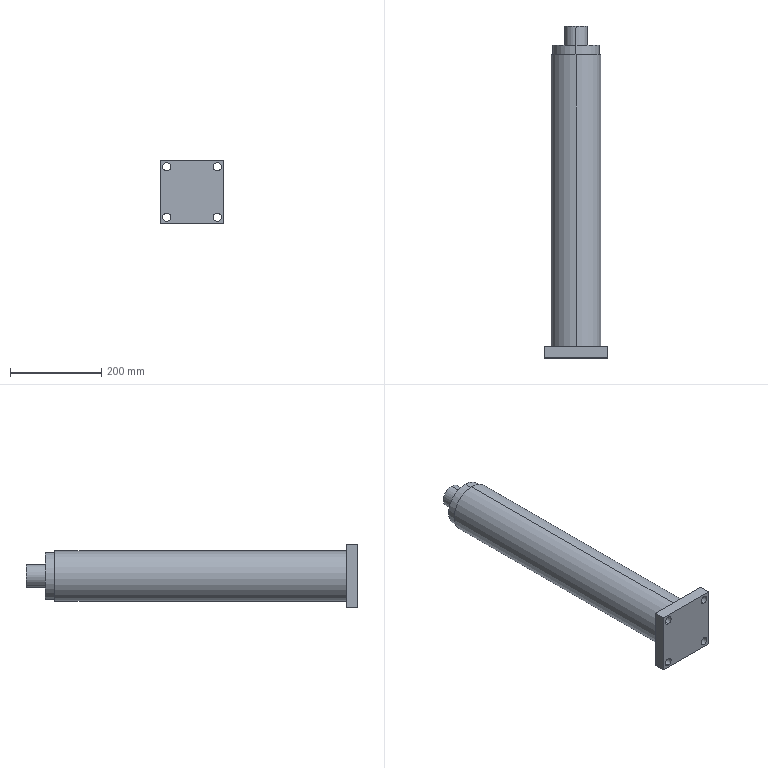Part | SolidWorks | features ICE 1, Revolution 1 | 1 solid | 23 faces | box 140 x 729 x 140 mm | volume 6809578 mm3 | cylinder 14 | plane 9 | commonest cylinder face diameters 18 x8 50 x2 102 x2 110 x2
STEP:
#1=CARTESIAN_POINT('',(-55.5,25.,46.5));
#2=VERTEX_POINT('',#1);
#3=CARTESIAN_POINT('',(-55.5,25.,64.5));
#4=VERTEX_POINT('',#3);
#5=CARTESIAN_POINT('',(-55.5,25.,55.5));
#6=DIRECTION('',(0.,1.,0.));
#7=DIRECTION('',(0.,0.,1.));
#8=AXIS2_PLACEMENT_3D('',#5,#6,#7);
#9=CIRCLE('',#8,9.);
#10=EDGE_CURVE('',#2,#4,#9,.T.);
#11=ORIENTED_EDGE('',*,*,#10,.T.);
#12=CARTESIAN_POINT('',(-55.5,0.,64.5));
#13=VERTEX_POINT('',#12);
#14=CARTESIAN_POINT('',(-55.5,25.,64.5));
#15=DIRECTION('',(0.,-1.,0.));
#16=VECTOR('',#15,1000.);
#17=LINE('',#14,#16);
#18=EDGE_CURVE('',#4,#13,#17,.T.);
#19=ORIENTED_EDGE('',*,*,#18,.T.);
#20=CARTESIAN_POINT('',(-55.5,0.,46.5));
#21=VERTEX_POINT('',#20);
#22=CARTESIAN_POINT('',(-55.5,0.,55.5));
#23=DIRECTION('',(0.,1.,0.));
#24=DIRECTION('',(0.,0.,1.));
#25=AXIS2_PLACEMENT_3D('',#22,#23,#24);
#26=CIRCLE('',#25,9.);
#27=EDGE_CURVE('',#21,#13,#26,.T.);
#28=ORIENTED_EDGE('',*,*,#27,.F.);
#29=CARTESIAN_POINT('',(-55.5,25.,46.5));
#30=DIRECTION('',(0.,-1.,0.));
#31=VECTOR('',#30,1000.);
#32=LINE('',#29,#31);
#33=EDGE_CURVE('',#2,#21,#32,.T.);
#34=ORIENTED_EDGE('',*,*,#33,.F.);
#35=EDGE_LOOP('',(#11,#19,#28,#34));
#36=FACE_OUTER_BOUND('',#35,.T.);
#37=CARTESIAN_POINT('',(-55.5,25.,55.5));
#38=DIRECTION('',(0.,-1.,0.));
#39=DIRECTION('',(0.,0.,-1.));
#40=AXIS2_PLACEMENT_3D('',#37,#38,#39);
#41=CYLINDRICAL_SURFACE('',#40,9.);
#42=ADVANCED_FACE('',(#36),#41,.F.);
#43=CARTESIAN_POINT('',(55.5,25.,46.5));
#44=VERTEX_POINT('',#43);
#45=CARTESIAN_POINT('',(55.5,25.,64.5));
#46=VERTEX_POINT('',#45);
#47=CARTESIAN_POINT('',(55.5,25.,55.5));
#48=DIRECTION('',(0.,1.,0.));
#49=DIRECTION('',(0.,0.,1.));
#50=AXIS2_PLACEMENT_3D('',#47,#48,#49);
#51=CIRCLE('',#50,9.);
#52=EDGE_CURVE('',#44,#46,#51,.T.);
#53=ORIENTED_EDGE('',*,*,#52,.T.);
#54=CARTESIAN_POINT('',(55.5,0.,64.5));
#55=VERTEX_POINT('',#54);
#56=CARTESIAN_POINT('',(55.5,25.,64.5));
#57=DIRECTION('',(0.,-1.,0.));
#58=VECTOR('',#57,1000.);
#59=LINE('',#56,#58);
#60=EDGE_CURVE('',#46,#55,#59,.T.);
#61=ORIENTED_EDGE('',*,*,#60,.T.);
#62=CARTESIAN_POINT('',(55.5,0.,46.5));
#63=VERTEX_POINT('',#62);
#64=CARTESIAN_POINT('',(55.5,0.,55.5));
#65=DIRECTION('',(0.,1.,0.));
#66=DIRECTION('',(0.,0.,1.));
#67=AXIS2_PLACEMENT_3D('',#64,#65,#66);
#68=CIRCLE('',#67,9.);
#69=EDGE_CURVE('',#63,#55,#68,.T.);
#70=ORIENTED_EDGE('',*,*,#69,.F.);
#71=CARTESIAN_POINT('',(55.5,25.,46.5));
#72=DIRECTION('',(0.,-1.,0.));
#73=VECTOR('',#72,1000.);
#74=LINE('',#71,#73);
#75=EDGE_CURVE('',#44,#63,#74,.T.);
#76=ORIENTED_EDGE('',*,*,#75,.F.);
#77=EDGE_LOOP('',(#53,#61,#70,#76));
#78=FACE_OUTER_BOUND('',#77,.T.);
#79=CARTESIAN_POINT('',(55.5,25.,55.5));
#80=DIRECTION('',(0.,-1.,0.));
#81=DIRECTION('',(0.,0.,-1.));
#82=AXIS2_PLACEMENT_3D('',#79,#80,#81);
#83=CYLINDRICAL_SURFACE('',#82,9.);
#84=ADVANCED_FACE('',(#78),#83,.F.);
#85=CARTESIAN_POINT('',(55.5,25.,-64.5));
#86=VERTEX_POINT('',#85);
#87=CARTESIAN_POINT('',(55.5,25.,-46.5));
#88=VERTEX_POINT('',#87);
#89=CARTESIAN_POINT('',(55.5,25.,-55.5));
#90=DIRECTION('',(0.,1.,0.));
#91=DIRECTION('',(0.,0.,1.));
#92=AXIS2_PLACEMENT_3D('',#89,#90,#91);
#93=CIRCLE('',#92,9.);
#94=EDGE_CURVE('',#86,#88,#93,.T.);
#95=ORIENTED_EDGE('',*,*,#94,.T.);
#96=CARTESIAN_POINT('',(55.5,0.,-46.5));
#97=VERTEX_POINT('',#96);
#98=CARTESIAN_POINT('',(55.5,25.,-46.5));
#99=DIRECTION('',(0.,-1.,0.));
#100=VECTOR('',#99,1000.);
#101=LINE('',#98,#100);
#102=EDGE_CURVE('',#88,#97,#101,.T.);
#103=ORIENTED_EDGE('',*,*,#102,.T.);
#104=CARTESIAN_POINT('',(55.5,0.,-64.5));
#105=VERTEX_POINT('',#104);
#106=CARTESIAN_POINT('',(55.5,0.,-55.5));
#107=DIRECTION('',(0.,1.,0.));
#108=DIRECTION('',(0.,0.,1.));
#109=AXIS2_PLACEMENT_3D('',#106,#107,#108);
#110=CIRCLE('',#109,9.);
#111=EDGE_CURVE('',#105,#97,#110,.T.);
#112=ORIENTED_EDGE('',*,*,#111,.F.);
#113=CARTESIAN_POINT('',(55.5,25.,-64.5));
#114=DIRECTION('',(0.,-1.,0.));
#115=VECTOR('',#114,1000.);
#116=LINE('',#113,#115);
#117=EDGE_CURVE('',#86,#105,#116,.T.);
#118=ORIENTED_EDGE('',*,*,#117,.F.);
#119=EDGE_LOOP('',(#95,#103,#112,#118));
#120=FACE_OUTER_BOUND('',#119,.T.);
#121=CARTESIAN_POINT('',(55.5,25.,-55.5));
#122=DIRECTION('',(0.,-1.,0.));
#123=DIRECTION('',(0.,0.,-1.));
#124=AXIS2_PLACEMENT_3D('',#121,#122,#123);
#125=CYLINDRICAL_SURFACE('',#124,9.);
#126=ADVANCED_FACE('',(#120),#125,.F.);
#127=CARTESIAN_POINT('',(-55.5,25.,-64.5));
#128=VERTEX_POINT('',#127);
#129=CARTESIAN_POINT('',(-55.5,25.,-46.5));
#130=VERTEX_POINT('',#129);
#131=CARTESIAN_POINT('',(-55.5,25.,-55.5));
#132=DIRECTION('',(0.,1.,0.));
#133=DIRECTION('',(0.,0.,1.));
#134=AXIS2_PLACEMENT_3D('',#131,#132,#133);
#135=CIRCLE('',#134,9.);
#136=EDGE_CURVE('',#128,#130,#135,.T.);
#137=ORIENTED_EDGE('',*,*,#136,.T.);
#138=CARTESIAN_POINT('',(-55.5,0.,-46.5));
#139=VERTEX_POINT('',#138);
#140=CARTESIAN_POINT('',(-55.5,25.,-46.5));
#141=DIRECTION('',(0.,-1.,0.));
#142=VECTOR('',#141,1000.);
#143=LINE('',#140,#142);
#144=EDGE_CURVE('',#130,#139,#143,.T.);
#145=ORIENTED_EDGE('',*,*,#144,.T.);
#146=CARTESIAN_POINT('',(-55.5,0.,-64.5));
#147=VERTEX_POINT('',#146);
#148=CARTESIAN_POINT('',(-55.5,0.,-55.5));
#149=DIRECTION('',(0.,1.,0.));
#150=DIRECTION('',(0.,0.,1.));
#151=AXIS2_PLACEMENT_3D('',#148,#149,#150);
#152=CIRCLE('',#151,9.);
#153=EDGE_CURVE('',#147,#139,#152,.T.);
#154=ORIENTED_EDGE('',*,*,#153,.F.);
#155=CARTESIAN_POINT('',(-55.5,25.,-64.5));
#156=DIRECTION('',(0.,-1.,0.));
#157=VECTOR('',#156,1000.);
#158=LINE('',#155,#157);
#159=EDGE_CURVE('',#128,#147,#158,.T.);
#160=ORIENTED_EDGE('',*,*,#159,.F.);
#161=EDGE_LOOP('',(#137,#145,#154,#160));
#162=FACE_OUTER_BOUND('',#161,.T.);
#163=CARTESIAN_POINT('',(-55.5,25.,-55.5));
#164=DIRECTION('',(0.,-1.,0.));
#165=DIRECTION('',(0.,0.,-1.));
#166=AXIS2_PLACEMENT_3D('',#163,#164,#165);
#167=CYLINDRICAL_SURFACE('',#166,9.);
#168=ADVANCED_FACE('',(#162),#167,.F.);
#169=CARTESIAN_POINT('',(0.,687.,25.));
#170=VERTEX_POINT('',#169);
#171=CARTESIAN_POINT('',(0.,687.,-25.));
#172=VERTEX_POINT('',#171);
#173=CARTESIAN_POINT('',(0.,687.,0.));
#174=DIRECTION('',(0.,1.,0.));
#175=DIRECTION('',(0.,0.,1.));
#176=AXIS2_PLACEMENT_3D('',#173,#174,#175);
#177=CIRCLE('',#176,25.);
#178=EDGE_CURVE('',#170,#172,#177,.T.);
#179=ORIENTED_EDGE('',*,*,#178,.T.);
#180=CARTESIAN_POINT('',(0.,729.,-25.));
#181=VERTEX_POINT('',#180);
#182=CARTESIAN_POINT('',(0.,0.,-25.));
#183=DIRECTION('',(0.,1.,0.));
#184=VECTOR('',#183,1000.);
#185=LINE('',#182,#184);
#186=EDGE_CURVE('',#172,#181,#185,.T.);
#187=ORIENTED_EDGE('',*,*,#186,.T.);
#188=CARTESIAN_POINT('',(0.,729.,25.));
#189=VERTEX_POINT('',#188);
#190=CARTESIAN_POINT('',(0.,729.,0.));
#191=DIRECTION('',(0.,1.,0.));
#192=DIRECTION('',(0.,0.,1.));
#193=AXIS2_PLACEMENT_3D('',#190,#191,#192);
#194=CIRCLE('',#193,25.);
#195=EDGE_CURVE('',#189,#181,#194,.T.);
#196=ORIENTED_EDGE('',*,*,#195,.F.);
#197=CARTESIAN_POINT('',(0.,0.,25.));
#198=DIRECTION('',(0.,1.,0.));
#199=VECTOR('',#198,1000.);
#200=LINE('',#197,#199);
#201=EDGE_CURVE('',#170,#189,#200,.T.);
#202=ORIENTED_EDGE('',*,*,#201,.F.);
#203=EDGE_LOOP('',(#179,#187,#196,#202));
#204=FACE_OUTER_BOUND('',#203,.T.);
#205=CARTESIAN_POINT('',(0.,0.,0.));
#206=DIRECTION('',(0.,1.,0.));
#207=DIRECTION('',(0.,0.,1.));
#208=AXIS2_PLACEMENT_3D('',#205,#206,#207);
#209=CYLINDRICAL_SURFACE('',#208,25.);
#210=ADVANCED_FACE('',(#204),#209,.T.);
#211=CARTESIAN_POINT('',(0.,665.5,51.));
#212=VERTEX_POINT('',#211);
#213=CARTESIAN_POINT('',(0.,665.5,-51.));
#214=VERTEX_POINT('',#213);
#215=CARTESIAN_POINT('',(0.,665.5,0.));
#216=DIRECTION('',(0.,1.,0.));
#217=DIRECTION('',(0.,0.,1.));
#218=AXIS2_PLACEMENT_3D('',#215,#216,#217);
#219=CIRCLE('',#218,51.);
#220=EDGE_CURVE('',#212,#214,#219,.T.);
#221=ORIENTED_EDGE('',*,*,#220,.T.);
#222=CARTESIAN_POINT('',(0.,687.,-51.));
#223=VERTEX_POINT('',#222);
#224=CARTESIAN_POINT('',(0.,0.,-51.));
#225=DIRECTION('',(0.,1.,0.));
#226=VECTOR('',#225,1000.);
#227=LINE('',#224,#226);
#228=EDGE_CURVE('',#214,#223,#227,.T.);
#229=ORIENTED_EDGE('',*,*,#228,.T.);
#230=CARTESIAN_POINT('',(0.,687.,51.));
#231=VERTEX_POINT('',#230);
#232=CARTESIAN_POINT('',(0.,687.,0.));
#233=DIRECTION('',(0.,1.,0.));
#234=DIRECTION('',(0.,0.,1.));
#235=AXIS2_PLACEMENT_3D('',#232,#233,#234);
#236=CIRCLE('',#235,51.);
#237=EDGE_CURVE('',#231,#223,#236,.T.);
#238=ORIENTED_EDGE('',*,*,#237,.F.);
#239=CARTESIAN_POINT('',(0.,0.,51.));
#240=DIRECTION('',(0.,1.,0.));
#241=VECTOR('',#240,1000.);
#242=LINE('',#239,#241);
#243=EDGE_CURVE('',#212,#231,#242,.T.);
#244=ORIENTED_EDGE('',*,*,#243,.F.);
#245=EDGE_LOOP('',(#221,#229,#238,#244));
#246=FACE_OUTER_BOUND('',#245,.T.);
#247=CARTESIAN_POINT('',(0.,0.,0.));
#248=DIRECTION('',(0.,1.,0.));
#249=DIRECTION('',(0.,0.,1.));
#250=AXIS2_PLACEMENT_3D('',#247,#248,#249);
#251=CYLINDRICAL_SURFACE('',#250,51.);
#252=ADVANCED_FACE('',(#246),#251,.T.);
#253=CARTESIAN_POINT('',(0.,25.,55.));
#254=VERTEX_POINT('',#253);
#255=CARTESIAN_POINT('',(0.,25.,-55.));
#256=VERTEX_POINT('',#255);
#257=CARTESIAN_POINT('',(0.,25.,0.));
#258=DIRECTION('',(0.,1.,0.));
#259=DIRECTION('',(0.,0.,1.));
#260=AXIS2_PLACEMENT_3D('',#257,#258,#259);
#261=CIRCLE('',#260,55.);
#262=EDGE_CURVE('',#254,#256,#261,.T.);
#263=ORIENTED_EDGE('',*,*,#262,.T.);
#264=CARTESIAN_POINT('',(0.,665.5,-55.));
#265=VERTEX_POINT('',#264);
#266=CARTESIAN_POINT('',(0.,0.,-55.));
#267=DIRECTION('',(0.,1.,0.));
#268=VECTOR('',#267,1000.);
#269=LINE('',#266,#268);
#270=EDGE_CURVE('',#256,#265,#269,.T.);
#271=ORIENTED_EDGE('',*,*,#270,.T.);
#272=CARTESIAN_POINT('',(0.,665.5,55.));
#273=VERTEX_POINT('',#272);
#274=CARTESIAN_POINT('',(0.,665.5,0.));
#275=DIRECTION('',(0.,1.,0.));
#276=DIRECTION('',(0.,0.,1.));
#277=AXIS2_PLACEMENT_3D('',#274,#275,#276);
#278=CIRCLE('',#277,55.);
#279=EDGE_CURVE('',#273,#265,#278,.T.);
#280=ORIENTED_EDGE('',*,*,#279,.F.);
#281=CARTESIAN_POINT('',(0.,0.,55.));
#282=DIRECTION('',(0.,1.,0.));
#283=VECTOR('',#282,1000.);
#284=LINE('',#281,#283);
#285=EDGE_CURVE('',#254,#273,#284,.T.);
#286=ORIENTED_EDGE('',*,*,#285,.F.);
#287=EDGE_LOOP('',(#263,#271,#280,#286));
#288=FACE_OUTER_BOUND('',#287,.T.);
#289=CARTESIAN_POINT('',(0.,0.,0.));
#290=DIRECTION('',(0.,1.,0.));
#291=DIRECTION('',(0.,0.,1.));
#292=AXIS2_PLACEMENT_3D('',#289,#290,#291);
#293=CYLINDRICAL_SURFACE('',#292,55.);
#294=ADVANCED_FACE('',(#288),#293,.T.);
#295=ORIENTED_EDGE('',*,*,#262,.F.);
#296=CARTESIAN_POINT('',(0.,25.,0.));
#297=DIRECTION('',(0.,1.,0.));
#298=DIRECTION('',(0.,0.,1.));
#299=AXIS2_PLACEMENT_3D('',#296,#297,#298);
#300=CIRCLE('',#299,55.);
#301=EDGE_CURVE('',#256,#254,#300,.T.);
#302=ORIENTED_EDGE('',*,*,#301,.F.);
#303=EDGE_LOOP('',(#295,#302));
#304=FACE_BOUND('',#303,.T.);
#305=ORIENTED_EDGE('',*,*,#52,.F.);
#306=CARTESIAN_POINT('',(55.5,25.,55.5));
#307=DIRECTION('',(0.,1.,0.));
#308=DIRECTION('',(0.,0.,1.));
#309=AXIS2_PLACEMENT_3D('',#306,#307,#308);
#310=CIRCLE('',#309,9.);
#311=EDGE_CURVE('',#46,#44,#310,.T.);
#312=ORIENTED_EDGE('',*,*,#311,.F.);
#313=EDGE_LOOP('',(#305,#312));
#314=FACE_BOUND('',#313,.T.);
#315=ORIENTED_EDGE('',*,*,#136,.F.);
#316=CARTESIAN_POINT('',(-55.5,25.,-55.5));
#317=DIRECTION('',(0.,1.,0.));
#318=DIRECTION('',(0.,0.,1.));
#319=AXIS2_PLACEMENT_3D('',#316,#317,#318);
#320=CIRCLE('',#319,9.);
#321=EDGE_CURVE('',#130,#128,#320,.T.);
#322=ORIENTED_EDGE('',*,*,#321,.F.);
#323=EDGE_LOOP('',(#315,#322));
#324=FACE_BOUND('',#323,.T.);
#325=CARTESIAN_POINT('',(-70.,25.,-70.));
#326=VERTEX_POINT('',#325);
#327=CARTESIAN_POINT('',(-70.,25.,70.));
#328=VERTEX_POINT('',#327);
#329=CARTESIAN_POINT('',(-70.,25.,70.));
#330=DIRECTION('',(0.,0.,1.));
#331=VECTOR('',#330,1000.);
#332=LINE('',#329,#331);
#333=EDGE_CURVE('',#326,#328,#332,.T.);
#334=ORIENTED_EDGE('',*,*,#333,.T.);
#335=CARTESIAN_POINT('',(70.,25.,70.));
#336=VERTEX_POINT('',#335);
#337=CARTESIAN_POINT('',(70.,25.,70.));
#338=DIRECTION('',(1.,0.,0.));
#339=VECTOR('',#338,1000.);
#340=LINE('',#337,#339);
#341=EDGE_CURVE('',#328,#336,#340,.T.);
#342=ORIENTED_EDGE('',*,*,#341,.T.);
#343=CARTESIAN_POINT('',(70.,25.,-70.));
#344=VERTEX_POINT('',#343);
#345=CARTESIAN_POINT('',(70.,25.,70.));
#346=DIRECTION('',(0.,0.,-1.));
#347=VECTOR('',#346,1000.);
#348=LINE('',#345,#347);
#349=EDGE_CURVE('',#336,#344,#348,.T.);
#350=ORIENTED_EDGE('',*,*,#349,.T.);
#351=CARTESIAN_POINT('',(70.,25.,-70.));
#352=DIRECTION('',(-1.,0.,0.));
#353=VECTOR('',#352,1000.);
#354=LINE('',#351,#353);
#355=EDGE_CURVE('',#344,#326,#354,.T.);
#356=ORIENTED_EDGE('',*,*,#355,.T.);
#357=EDGE_LOOP('',(#334,#342,#350,#356));
#358=FACE_OUTER_BOUND('',#357,.T.);
#359=ORIENTED_EDGE('',*,*,#94,.F.);
#360=CARTESIAN_POINT('',(55.5,25.,-55.5));
#361=DIRECTION('',(0.,1.,0.));
#362=DIRECTION('',(0.,0.,1.));
#363=AXIS2_PLACEMENT_3D('',#360,#361,#362);
#364=CIRCLE('',#363,9.);
#365=EDGE_CURVE('',#88,#86,#364,.T.);
#366=ORIENTED_EDGE('',*,*,#365,.F.);
#367=EDGE_LOOP('',(#359,#366));
#368=FACE_BOUND('',#367,.T.);
#369=ORIENTED_EDGE('',*,*,#10,.F.);
#370=CARTESIAN_POINT('',(-55.5,25.,55.5));
#371=DIRECTION('',(0.,1.,0.));
#372=DIRECTION('',(0.,0.,1.));
#373=AXIS2_PLACEMENT_3D('',#370,#371,#372);
#374=CIRCLE('',#373,9.);
#375=EDGE_CURVE('',#4,#2,#374,.T.);
#376=ORIENTED_EDGE('',*,*,#375,.F.);
#377=EDGE_LOOP('',(#369,#376));
#378=FACE_BOUND('',#377,.T.);
#379=CARTESIAN_POINT('',(60.,25.,0.));
#380=DIRECTION('',(0.,-1.,0.));
#381=DIRECTION('',(0.,0.,-1.));
#382=AXIS2_PLACEMENT_3D('',#379,#380,#381);
#383=PLANE('',#382);
#384=ADVANCED_FACE('',(#304,#314,#324,#358,#368,#378),#383,.F.);
#385=ORIENTED_EDGE('',*,*,#270,.F.);
#386=ORIENTED_EDGE('',*,*,#301,.T.);
#387=ORIENTED_EDGE('',*,*,#285,.T.);
#388=CARTESIAN_POINT('',(0.,665.5,0.));
#389=DIRECTION('',(0.,1.,0.));
#390=DIRECTION('',(0.,0.,1.));
#391=AXIS2_PLACEMENT_3D('',#388,#389,#390);
#392=CIRCLE('',#391,55.);
#393=EDGE_CURVE('',#265,#273,#392,.T.);
#394=ORIENTED_EDGE('',*,*,#393,.F.);
#395=EDGE_LOOP('',(#385,#386,#387,#394));
#396=FACE_OUTER_BOUND('',#395,.T.);
#397=CARTESIAN_POINT('',(0.,0.,0.));
#398=DIRECTION('',(0.,1.,0.));
#399=DIRECTION('',(0.,0.,1.));
#400=AXIS2_PLACEMENT_3D('',#397,#398,#399);
#401=CYLINDRICAL_SURFACE('',#400,55.);
#402=ADVANCED_FACE('',(#396),#401,.T.);
#403=ORIENTED_EDGE('',*,*,#220,.F.);
#404=CARTESIAN_POINT('',(0.,665.5,0.));
#405=DIRECTION('',(0.,1.,0.));
#406=DIRECTION('',(0.,0.,1.));
#407=AXIS2_PLACEMENT_3D('',#404,#405,#406);
#408=CIRCLE('',#407,51.);
#409=EDGE_CURVE('',#214,#212,#408,.T.);
#410=ORIENTED_EDGE('',*,*,#409,.F.);
#411=EDGE_LOOP('',(#403,#410));
#412=FACE_BOUND('',#411,.T.);
#413=ORIENTED_EDGE('',*,*,#279,.T.);
#414=ORIENTED_EDGE('',*,*,#393,.T.);
#415=EDGE_LOOP('',(#413,#414));
#416=FACE_OUTER_BOUND('',#415,.T.);
#417=CARTESIAN_POINT('',(55.,665.5,0.));
#418=DIRECTION('',(0.,-1.,0.));
#419=DIRECTION('',(0.,0.,-1.));
#420=AXIS2_PLACEMENT_3D('',#417,#418,#419);
#421=PLANE('',#420);
#422=ADVANCED_FACE('',(#412,#416),#421,.F.);
#423=ORIENTED_EDGE('',*,*,#228,.F.);
#424=ORIENTED_EDGE('',*,*,#409,.T.);
#425=ORIENTED_EDGE('',*,*,#243,.T.);
#426=CARTESIAN_POINT('',(0.,687.,0.));
#427=DIRECTION('',(0.,1.,0.));
#428=DIRECTION('',(0.,0.,1.));
#429=AXIS2_PLACEMENT_3D('',#426,#427,#428);
#430=CIRCLE('',#429,51.);
#431=EDGE_CURVE('',#223,#231,#430,.T.);
#432=ORIENTED_EDGE('',*,*,#431,.F.);
#433=EDGE_LOOP('',(#423,#424,#425,#432));
#434=FACE_OUTER_BOUND('',#433,.T.);
#435=CARTESIAN_POINT('',(0.,0.,0.));
#436=DIRECTION('',(0.,1.,0.));
#437=DIRECTION('',(0.,0.,1.));
#438=AXIS2_PLACEMENT_3D('',#435,#436,#437);
#439=CYLINDRICAL_SURFACE('',#438,51.);
#440=ADVANCED_FACE('',(#434),#439,.T.);
#441=ORIENTED_EDGE('',*,*,#178,.F.);
#442=CARTESIAN_POINT('',(0.,687.,0.));
#443=DIRECTION('',(0.,1.,0.));
#444=DIRECTION('',(0.,0.,1.));
#445=AXIS2_PLACEMENT_3D('',#442,#443,#444);
#446=CIRCLE('',#445,25.);
#447=EDGE_CURVE('',#172,#170,#446,.T.);
#448=ORIENTED_EDGE('',*,*,#447,.F.);
#449=EDGE_LOOP('',(#441,#448));
#450=FACE_BOUND('',#449,.T.);
#451=ORIENTED_EDGE('',*,*,#237,.T.);
#452=ORIENTED_EDGE('',*,*,#431,.T.);
#453=EDGE_LOOP('',(#451,#452));
#454=FACE_OUTER_BOUND('',#453,.T.);
#455=CARTESIAN_POINT('',(51.,687.,0.));
#456=DIRECTION('',(0.,-1.,0.));
#457=DIRECTION('',(0.,0.,-1.));
#458=AXIS2_PLACEMENT_3D('',#455,#456,#457);
#459=PLANE('',#458);
#460=ADVANCED_FACE('',(#450,#454),#459,.F.);
#461=ORIENTED_EDGE('',*,*,#186,.F.);
#462=ORIENTED_EDGE('',*,*,#447,.T.);
#463=ORIENTED_EDGE('',*,*,#201,.T.);
#464=CARTESIAN_POINT('',(0.,729.,0.));
#465=DIRECTION('',(0.,1.,0.));
#466=DIRECTION('',(0.,0.,1.));
#467=AXIS2_PLACEMENT_3D('',#464,#465,#466);
#468=CIRCLE('',#467,25.);
#469=EDGE_CURVE('',#181,#189,#468,.T.);
#470=ORIENTED_EDGE('',*,*,#469,.F.);
#471=EDGE_LOOP('',(#461,#462,#463,#470));
#472=FACE_OUTER_BOUND('',#471,.T.);
#473=CARTESIAN_POINT('',(0.,0.,0.));
#474=DIRECTION('',(0.,1.,0.));
#475=DIRECTION('',(0.,0.,1.));
#476=AXIS2_PLACEMENT_3D('',#473,#474,#475);
#477=CYLINDRICAL_SURFACE('',#476,25.);
#478=ADVANCED_FACE('',(#472),#477,.T.);
#479=ORIENTED_EDGE('',*,*,#195,.T.);
#480=ORIENTED_EDGE('',*,*,#469,.T.);
#481=EDGE_LOOP('',(#479,#480));
#482=FACE_OUTER_BOUND('',#481,.T.);
#483=CARTESIAN_POINT('',(25.,729.,0.));
#484=DIRECTION('',(0.,-1.,0.));
#485=DIRECTION('',(0.,0.,-1.));
#486=AXIS2_PLACEMENT_3D('',#483,#484,#485);
#487=PLANE('',#486);
#488=ADVANCED_FACE('',(#482),#487,.F.);
#489=CARTESIAN_POINT('',(-70.,0.,-70.));
#490=VERTEX_POINT('',#489);
#491=CARTESIAN_POINT('',(-70.,0.,70.));
#492=VERTEX_POINT('',#491);
#493=CARTESIAN_POINT('',(-70.,0.,70.));
#494=DIRECTION('',(0.,0.,1.));
#495=VECTOR('',#494,1000.);
#496=LINE('',#493,#495);
#497=EDGE_CURVE('',#490,#492,#496,.T.);
#498=ORIENTED_EDGE('',*,*,#497,.T.);
#499=CARTESIAN_POINT('',(-70.,25.,70.));
#500=DIRECTION('',(0.,-1.,0.));
#501=VECTOR('',#500,1000.);
#502=LINE('',#499,#501);
#503=EDGE_CURVE('',#328,#492,#502,.T.);
#504=ORIENTED_EDGE('',*,*,#503,.F.);
#505=ORIENTED_EDGE('',*,*,#333,.F.);
#506=CARTESIAN_POINT('',(-70.,25.,-70.));
#507=DIRECTION('',(0.,-1.,0.));
#508=VECTOR('',#507,1000.);
#509=LINE('',#506,#508);
#510=EDGE_CURVE('',#326,#490,#509,.T.);
#511=ORIENTED_EDGE('',*,*,#510,.T.);
#512=EDGE_LOOP('',(#498,#504,#505,#511));
#513=FACE_OUTER_BOUND('',#512,.T.);
#514=CARTESIAN_POINT('',(-70.,25.,70.));
#515=DIRECTION('',(1.,0.,0.));
#516=DIRECTION('',(0.,0.,-1.));
#517=AXIS2_PLACEMENT_3D('',#514,#515,#516);
#518=PLANE('',#517);
#519=ADVANCED_FACE('',(#513),#518,.F.);
#520=CARTESIAN_POINT('',(70.,0.,70.));
#521=VERTEX_POINT('',#520);
#522=CARTESIAN_POINT('',(70.,0.,70.));
#523=DIRECTION('',(1.,0.,0.));
#524=VECTOR('',#523,1000.);
#525=LINE('',#522,#524);
#526=EDGE_CURVE('',#492,#521,#525,.T.);
#527=ORIENTED_EDGE('',*,*,#526,.T.);
#528=CARTESIAN_POINT('',(70.,25.,70.));
#529=DIRECTION('',(0.,-1.,0.));
#530=VECTOR('',#529,1000.);
#531=LINE('',#528,#530);
#532=EDGE_CURVE('',#336,#521,#531,.T.);
#533=ORIENTED_EDGE('',*,*,#532,.F.);
#534=ORIENTED_EDGE('',*,*,#341,.F.);
#535=ORIENTED_EDGE('',*,*,#503,.T.);
#536=EDGE_LOOP('',(#527,#533,#534,#535));
#537=FACE_OUTER_BOUND('',#536,.T.);
#538=CARTESIAN_POINT('',(70.,25.,70.));
#539=DIRECTION('',(0.,0.,-1.));
#540=DIRECTION('',(-1.,0.,0.));
#541=AXIS2_PLACEMENT_3D('',#538,#539,#540);
#542=PLANE('',#541);
#543=ADVANCED_FACE('',(#537),#542,.F.);
#544=CARTESIAN_POINT('',(70.,0.,-70.));
#545=VERTEX_POINT('',#544);
#546=CARTESIAN_POINT('',(70.,0.,70.));
#547=DIRECTION('',(0.,0.,-1.));
#548=VECTOR('',#547,1000.);
#549=LINE('',#546,#548);
#550=EDGE_CURVE('',#521,#545,#549,.T.);
#551=ORIENTED_EDGE('',*,*,#550,.T.);
#552=CARTESIAN_POINT('',(70.,25.,-70.));
#553=DIRECTION('',(0.,-1.,0.));
#554=VECTOR('',#553,1000.);
#555=LINE('',#552,#554);
#556=EDGE_CURVE('',#344,#545,#555,.T.);
#557=ORIENTED_EDGE('',*,*,#556,.F.);
#558=ORIENTED_EDGE('',*,*,#349,.F.);
#559=ORIENTED_EDGE('',*,*,#532,.T.);
#560=EDGE_LOOP('',(#551,#557,#558,#559));
#561=FACE_OUTER_BOUND('',#560,.T.);
#562=CARTESIAN_POINT('',(70.,25.,70.));
#563=DIRECTION('',(-1.,0.,0.));
#564=DIRECTION('',(0.,0.,1.));
#565=AXIS2_PLACEMENT_3D('',#562,#563,#564);
#566=PLANE('',#565);
#567=ADVANCED_FACE('',(#561),#566,.F.);
#568=CARTESIAN_POINT('',(70.,0.,-70.));
#569=DIRECTION('',(-1.,0.,0.));
#570=VECTOR('',#569,1000.);
#571=LINE('',#568,#570);
#572=EDGE_CURVE('',#545,#490,#571,.T.);
#573=ORIENTED_EDGE('',*,*,#572,.T.);
#574=ORIENTED_EDGE('',*,*,#510,.F.);
#575=ORIENTED_EDGE('',*,*,#355,.F.);
#576=ORIENTED_EDGE('',*,*,#556,.T.);
#577=EDGE_LOOP('',(#573,#574,#575,#576));
#578=FACE_OUTER_BOUND('',#577,.T.);
#579=CARTESIAN_POINT('',(70.,25.,-70.));
#580=DIRECTION('',(0.,0.,1.));
#581=DIRECTION('',(1.,0.,0.));
#582=AXIS2_PLACEMENT_3D('',#579,#580,#581);
#583=PLANE('',#582);
#584=ADVANCED_FACE('',(#578),#583,.F.);
#585=ORIENTED_EDGE('',*,*,#144,.F.);
#586=ORIENTED_EDGE('',*,*,#321,.T.);
#587=ORIENTED_EDGE('',*,*,#159,.T.);
#588=CARTESIAN_POINT('',(-55.5,0.,-55.5));
#589=DIRECTION('',(0.,1.,0.));
#590=DIRECTION('',(0.,0.,1.));
#591=AXIS2_PLACEMENT_3D('',#588,#589,#590);
#592=CIRCLE('',#591,9.);
#593=EDGE_CURVE('',#139,#147,#592,.T.);
#594=ORIENTED_EDGE('',*,*,#593,.F.);
#595=EDGE_LOOP('',(#585,#586,#587,#594));
#596=FACE_OUTER_BOUND('',#595,.T.);
#597=CARTESIAN_POINT('',(-55.5,25.,-55.5));
#598=DIRECTION('',(0.,-1.,0.));
#599=DIRECTION('',(0.,0.,-1.));
#600=AXIS2_PLACEMENT_3D('',#597,#598,#599);
#601=CYLINDRICAL_SURFACE('',#600,9.);
#602=ADVANCED_FACE('',(#596),#601,.F.);
#603=ORIENTED_EDGE('',*,*,#102,.F.);
#604=ORIENTED_EDGE('',*,*,#365,.T.);
#605=ORIENTED_EDGE('',*,*,#117,.T.);
#606=CARTESIAN_POINT('',(55.5,0.,-55.5));
#607=DIRECTION('',(0.,1.,0.));
#608=DIRECTION('',(0.,0.,1.));
#609=AXIS2_PLACEMENT_3D('',#606,#607,#608);
#610=CIRCLE('',#609,9.);
#611=EDGE_CURVE('',#97,#105,#610,.T.);
#612=ORIENTED_EDGE('',*,*,#611,.F.);
#613=EDGE_LOOP('',(#603,#604,#605,#612));
#614=FACE_OUTER_BOUND('',#613,.T.);
#615=CARTESIAN_POINT('',(55.5,25.,-55.5));
#616=DIRECTION('',(0.,-1.,0.));
#617=DIRECTION('',(0.,0.,-1.));
#618=AXIS2_PLACEMENT_3D('',#615,#616,#617);
#619=CYLINDRICAL_SURFACE('',#618,9.);
#620=ADVANCED_FACE('',(#614),#619,.F.);
#621=ORIENTED_EDGE('',*,*,#60,.F.);
#622=ORIENTED_EDGE('',*,*,#311,.T.);
#623=ORIENTED_EDGE('',*,*,#75,.T.);
#624=CARTESIAN_POINT('',(55.5,0.,55.5));
#625=DIRECTION('',(0.,1.,0.));
#626=DIRECTION('',(0.,0.,1.));
#627=AXIS2_PLACEMENT_3D('',#624,#625,#626);
#628=CIRCLE('',#627,9.);
#629=EDGE_CURVE('',#55,#63,#628,.T.);
#630=ORIENTED_EDGE('',*,*,#629,.F.);
#631=EDGE_LOOP('',(#621,#622,#623,#630));
#632=FACE_OUTER_BOUND('',#631,.T.);
#633=CARTESIAN_POINT('',(55.5,25.,55.5));
#634=DIRECTION('',(0.,-1.,0.));
#635=DIRECTION('',(0.,0.,-1.));
#636=AXIS2_PLACEMENT_3D('',#633,#634,#635);
#637=CYLINDRICAL_SURFACE('',#636,9.);
#638=ADVANCED_FACE('',(#632),#637,.F.);
#639=ORIENTED_EDGE('',*,*,#18,.F.);
#640=ORIENTED_EDGE('',*,*,#375,.T.);
#641=ORIENTED_EDGE('',*,*,#33,.T.);
#642=CARTESIAN_POINT('',(-55.5,0.,55.5));
#643=DIRECTION('',(0.,1.,0.));
#644=DIRECTION('',(0.,0.,1.));
#645=AXIS2_PLACEMENT_3D('',#642,#643,#644);
#646=CIRCLE('',#645,9.);
#647=EDGE_CURVE('',#13,#21,#646,.T.);
#648=ORIENTED_EDGE('',*,*,#647,.F.);
#649=EDGE_LOOP('',(#639,#640,#641,#648));
#650=FACE_OUTER_BOUND('',#649,.T.);
#651=CARTESIAN_POINT('',(-55.5,25.,55.5));
#652=DIRECTION('',(0.,-1.,0.));
#653=DIRECTION('',(0.,0.,-1.));
#654=AXIS2_PLACEMENT_3D('',#651,#652,#653);
#655=CYLINDRICAL_SURFACE('',#654,9.);
#656=ADVANCED_FACE('',(#650),#655,.F.);
#657=ORIENTED_EDGE('',*,*,#497,.F.);
#658=ORIENTED_EDGE('',*,*,#572,.F.);
#659=ORIENTED_EDGE('',*,*,#550,.F.);
#660=ORIENTED_EDGE('',*,*,#526,.F.);
#661=EDGE_LOOP('',(#657,#658,#659,#660));
#662=FACE_OUTER_BOUND('',#661,.T.);
#663=ORIENTED_EDGE('',*,*,#153,.T.);
#664=ORIENTED_EDGE('',*,*,#593,.T.);
#665=EDGE_LOOP('',(#663,#664));
#666=FACE_BOUND('',#665,.T.);
#667=ORIENTED_EDGE('',*,*,#111,.T.);
#668=ORIENTED_EDGE('',*,*,#611,.T.);
#669=EDGE_LOOP('',(#667,#668));
#670=FACE_BOUND('',#669,.T.);
#671=ORIENTED_EDGE('',*,*,#69,.T.);
#672=ORIENTED_EDGE('',*,*,#629,.T.);
#673=EDGE_LOOP('',(#671,#672));
#674=FACE_BOUND('',#673,.T.);
#675=ORIENTED_EDGE('',*,*,#27,.T.);
#676=ORIENTED_EDGE('',*,*,#647,.T.);
#677=EDGE_LOOP('',(#675,#676));
#678=FACE_BOUND('',#677,.T.);
#679=CARTESIAN_POINT('',(0.,0.,0.));
#680=DIRECTION('',(0.,1.,0.));
#681=DIRECTION('',(0.,0.,1.));
#682=AXIS2_PLACEMENT_3D('',#679,#680,#681);
#683=PLANE('',#682);
#684=ADVANCED_FACE('',(#662,#666,#670,#674,#678),#683,.F.);
#685=CLOSED_SHELL('',(#42,#84,#126,#168,#210,#252,#294,#384,#402,#422,#440,#460,#478,#488,#519,#543,#567,#584,#602,#620,#638,#656,#684));
#686=MANIFOLD_SOLID_BREP('',#685);
#687=CARTESIAN_POINT('',(0.,0.,0.));
#688=DIRECTION('',(0.,0.,1.));
#689=DIRECTION('',(1.,0.,0.));
#690=AXIS2_PLACEMENT_3D('',#687,#688,#689);
#691=(LENGTH_UNIT()NAMED_UNIT(*)SI_UNIT(.MILLI.,.METRE.));
#692=UNCERTAINTY_MEASURE_WITH_UNIT(LENGTH_MEASURE(0.00001),#691,'','');
#693=(NAMED_UNIT(*)PLANE_ANGLE_UNIT()SI_UNIT($,.RADIAN.));
#694=(NAMED_UNIT(*)SI_UNIT($,.STERADIAN.)SOLID_ANGLE_UNIT());
#695=(GEOMETRIC_REPRESENTATION_CONTEXT(3)GLOBAL_UNCERTAINTY_ASSIGNED_CONTEXT((#692))GLOBAL_UNIT_ASSIGNED_CONTEXT((#691,#693,#694))REPRESENTATION_CONTEXT('',''));
#696=ADVANCED_BREP_SHAPE_REPRESENTATION('',(#686,#690),#695);